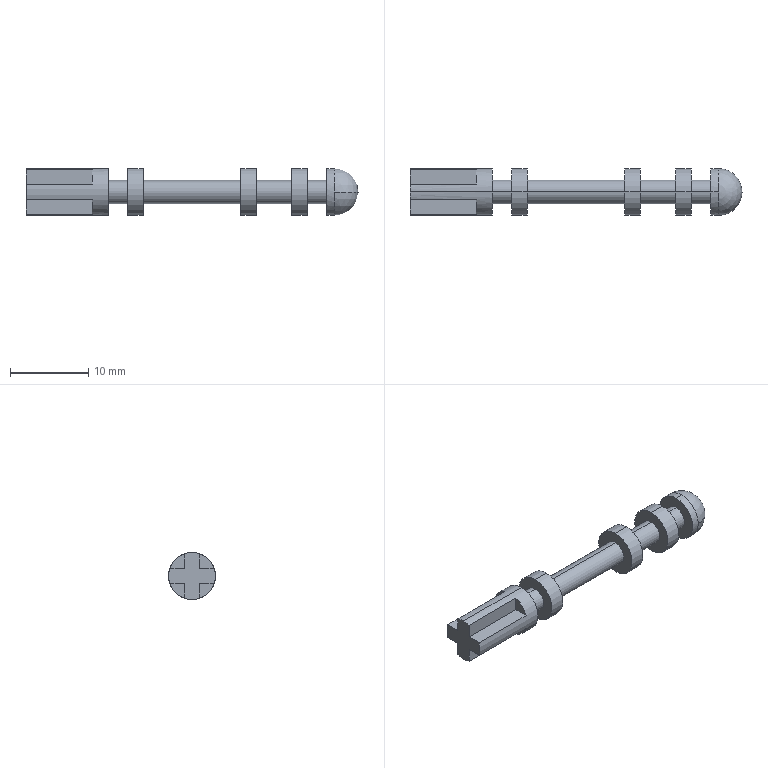Part | SolidWorks | features ICE 1, Revolution 1 | 1 solid | 41 faces | box 42.5 x 6 x 6 mm | volume 632.683 mm3 | plane 21 | cylinder 18 | sphere 2 | commonest cylinder face diameters 6 x10 3 x8
STEP:
#1=CARTESIAN_POINT('',(42.5,0.,0.));
#2=VERTEX_POINT('',#1);
#3=CARTESIAN_POINT('',(39.5,3.,0.));
#4=VERTEX_POINT('',#3);
#5=CARTESIAN_POINT('',(39.5,0.,0.));
#6=DIRECTION('',(0.,0.,1.));
#7=DIRECTION('',(1.,0.,0.));
#8=AXIS2_PLACEMENT_3D('',#5,#6,#7);
#9=CIRCLE('',#8,3.);
#10=EDGE_CURVE('',#2,#4,#9,.T.);
#11=ORIENTED_EDGE('',*,*,#10,.F.);
#12=CARTESIAN_POINT('',(39.5,-3.,0.));
#13=VERTEX_POINT('',#12);
#14=CARTESIAN_POINT('',(39.5,0.,0.));
#15=DIRECTION('',(0.,0.,-1.));
#16=DIRECTION('',(0.,1.,0.));
#17=AXIS2_PLACEMENT_3D('',#14,#15,#16);
#18=CIRCLE('',#17,3.);
#19=EDGE_CURVE('',#2,#13,#18,.T.);
#20=ORIENTED_EDGE('',*,*,#19,.T.);
#21=CARTESIAN_POINT('',(39.5,0.,-3.));
#22=VERTEX_POINT('',#21);
#23=CARTESIAN_POINT('',(39.5,0.,0.));
#24=DIRECTION('',(-1.,0.,0.));
#25=DIRECTION('',(0.,0.,1.));
#26=AXIS2_PLACEMENT_3D('',#23,#24,#25);
#27=CIRCLE('',#26,3.);
#28=EDGE_CURVE('',#22,#13,#27,.T.);
#29=ORIENTED_EDGE('',*,*,#28,.F.);
#30=CARTESIAN_POINT('',(39.5,0.,0.));
#31=DIRECTION('',(-1.,0.,0.));
#32=DIRECTION('',(0.,0.,1.));
#33=AXIS2_PLACEMENT_3D('',#30,#31,#32);
#34=CIRCLE('',#33,3.);
#35=EDGE_CURVE('',#4,#22,#34,.T.);
#36=ORIENTED_EDGE('',*,*,#35,.F.);
#37=EDGE_LOOP('',(#11,#20,#29,#36));
#38=FACE_OUTER_BOUND('',#37,.T.);
#39=CARTESIAN_POINT('',(39.5,0.,0.));
#40=DIRECTION('',(0.,0.,-1.));
#41=DIRECTION('',(0.,1.,0.));
#42=AXIS2_PLACEMENT_3D('',#39,#40,#41);
#43=SPHERICAL_SURFACE('',#42,3.);
#44=ADVANCED_FACE('',(#38),#43,.T.);
#45=CARTESIAN_POINT('',(39.5,0.,3.));
#46=VERTEX_POINT('',#45);
#47=CARTESIAN_POINT('',(39.5,0.,0.));
#48=DIRECTION('',(-1.,0.,0.));
#49=DIRECTION('',(0.,0.,1.));
#50=AXIS2_PLACEMENT_3D('',#47,#48,#49);
#51=CIRCLE('',#50,3.);
#52=EDGE_CURVE('',#46,#4,#51,.T.);
#53=ORIENTED_EDGE('',*,*,#52,.T.);
#54=ORIENTED_EDGE('',*,*,#35,.T.);
#55=CARTESIAN_POINT('',(38.5,0.,-3.));
#56=VERTEX_POINT('',#55);
#57=CARTESIAN_POINT('',(0.,0.,-3.));
#58=DIRECTION('',(-1.,0.,0.));
#59=VECTOR('',#58,1000.);
#60=LINE('',#57,#59);
#61=EDGE_CURVE('',#22,#56,#60,.T.);
#62=ORIENTED_EDGE('',*,*,#61,.T.);
#63=CARTESIAN_POINT('',(38.5,0.,3.));
#64=VERTEX_POINT('',#63);
#65=CARTESIAN_POINT('',(38.5,0.,0.));
#66=DIRECTION('',(-1.,0.,0.));
#67=DIRECTION('',(0.,0.,1.));
#68=AXIS2_PLACEMENT_3D('',#65,#66,#67);
#69=CIRCLE('',#68,3.);
#70=EDGE_CURVE('',#64,#56,#69,.T.);
#71=ORIENTED_EDGE('',*,*,#70,.F.);
#72=CARTESIAN_POINT('',(0.,0.,3.));
#73=DIRECTION('',(-1.,0.,0.));
#74=VECTOR('',#73,1000.);
#75=LINE('',#72,#74);
#76=EDGE_CURVE('',#46,#64,#75,.T.);
#77=ORIENTED_EDGE('',*,*,#76,.F.);
#78=EDGE_LOOP('',(#53,#54,#62,#71,#77));
#79=FACE_OUTER_BOUND('',#78,.T.);
#80=CARTESIAN_POINT('',(0.,0.,0.));
#81=DIRECTION('',(-1.,0.,0.));
#82=DIRECTION('',(0.,0.,1.));
#83=AXIS2_PLACEMENT_3D('',#80,#81,#82);
#84=CYLINDRICAL_SURFACE('',#83,3.);
#85=ADVANCED_FACE('',(#79),#84,.T.);
#86=CARTESIAN_POINT('',(38.5,0.,1.5));
#87=VERTEX_POINT('',#86);
#88=CARTESIAN_POINT('',(38.5,0.,-1.5));
#89=VERTEX_POINT('',#88);
#90=CARTESIAN_POINT('',(38.5,0.,0.));
#91=DIRECTION('',(-1.,0.,0.));
#92=DIRECTION('',(0.,0.,1.));
#93=AXIS2_PLACEMENT_3D('',#90,#91,#92);
#94=CIRCLE('',#93,1.5);
#95=EDGE_CURVE('',#87,#89,#94,.T.);
#96=ORIENTED_EDGE('',*,*,#95,.T.);
#97=CARTESIAN_POINT('',(36.,0.,-1.5));
#98=VERTEX_POINT('',#97);
#99=CARTESIAN_POINT('',(0.,0.,-1.5));
#100=DIRECTION('',(-1.,0.,0.));
#101=VECTOR('',#100,1000.);
#102=LINE('',#99,#101);
#103=EDGE_CURVE('',#89,#98,#102,.T.);
#104=ORIENTED_EDGE('',*,*,#103,.T.);
#105=CARTESIAN_POINT('',(36.,0.,1.5));
#106=VERTEX_POINT('',#105);
#107=CARTESIAN_POINT('',(36.,0.,0.));
#108=DIRECTION('',(-1.,0.,0.));
#109=DIRECTION('',(0.,0.,1.));
#110=AXIS2_PLACEMENT_3D('',#107,#108,#109);
#111=CIRCLE('',#110,1.5);
#112=EDGE_CURVE('',#106,#98,#111,.T.);
#113=ORIENTED_EDGE('',*,*,#112,.F.);
#114=CARTESIAN_POINT('',(0.,0.,1.5));
#115=DIRECTION('',(-1.,0.,0.));
#116=VECTOR('',#115,1000.);
#117=LINE('',#114,#116);
#118=EDGE_CURVE('',#87,#106,#117,.T.);
#119=ORIENTED_EDGE('',*,*,#118,.F.);
#120=EDGE_LOOP('',(#96,#104,#113,#119));
#121=FACE_OUTER_BOUND('',#120,.T.);
#122=CARTESIAN_POINT('',(0.,0.,0.));
#123=DIRECTION('',(-1.,0.,0.));
#124=DIRECTION('',(0.,0.,1.));
#125=AXIS2_PLACEMENT_3D('',#122,#123,#124);
#126=CYLINDRICAL_SURFACE('',#125,1.5);
#127=ADVANCED_FACE('',(#121),#126,.T.);
#128=CARTESIAN_POINT('',(36.,0.,3.));
#129=VERTEX_POINT('',#128);
#130=CARTESIAN_POINT('',(36.,0.,-3.));
#131=VERTEX_POINT('',#130);
#132=CARTESIAN_POINT('',(36.,0.,0.));
#133=DIRECTION('',(-1.,0.,0.));
#134=DIRECTION('',(0.,0.,1.));
#135=AXIS2_PLACEMENT_3D('',#132,#133,#134);
#136=CIRCLE('',#135,3.);
#137=EDGE_CURVE('',#129,#131,#136,.T.);
#138=ORIENTED_EDGE('',*,*,#137,.T.);
#139=CARTESIAN_POINT('',(34.,0.,-3.));
#140=VERTEX_POINT('',#139);
#141=CARTESIAN_POINT('',(0.,0.,-3.));
#142=DIRECTION('',(-1.,0.,0.));
#143=VECTOR('',#142,1000.);
#144=LINE('',#141,#143);
#145=EDGE_CURVE('',#131,#140,#144,.T.);
#146=ORIENTED_EDGE('',*,*,#145,.T.);
#147=CARTESIAN_POINT('',(34.,0.,3.));
#148=VERTEX_POINT('',#147);
#149=CARTESIAN_POINT('',(34.,0.,0.));
#150=DIRECTION('',(-1.,0.,0.));
#151=DIRECTION('',(0.,0.,1.));
#152=AXIS2_PLACEMENT_3D('',#149,#150,#151);
#153=CIRCLE('',#152,3.);
#154=EDGE_CURVE('',#148,#140,#153,.T.);
#155=ORIENTED_EDGE('',*,*,#154,.F.);
#156=CARTESIAN_POINT('',(0.,0.,3.));
#157=DIRECTION('',(-1.,0.,0.));
#158=VECTOR('',#157,1000.);
#159=LINE('',#156,#158);
#160=EDGE_CURVE('',#129,#148,#159,.T.);
#161=ORIENTED_EDGE('',*,*,#160,.F.);
#162=EDGE_LOOP('',(#138,#146,#155,#161));
#163=FACE_OUTER_BOUND('',#162,.T.);
#164=CARTESIAN_POINT('',(0.,0.,0.));
#165=DIRECTION('',(-1.,0.,0.));
#166=DIRECTION('',(0.,0.,1.));
#167=AXIS2_PLACEMENT_3D('',#164,#165,#166);
#168=CYLINDRICAL_SURFACE('',#167,3.);
#169=ADVANCED_FACE('',(#163),#168,.T.);
#170=CARTESIAN_POINT('',(34.,0.,1.5));
#171=VERTEX_POINT('',#170);
#172=CARTESIAN_POINT('',(34.,0.,-1.5));
#173=VERTEX_POINT('',#172);
#174=CARTESIAN_POINT('',(34.,0.,0.));
#175=DIRECTION('',(-1.,0.,0.));
#176=DIRECTION('',(0.,0.,1.));
#177=AXIS2_PLACEMENT_3D('',#174,#175,#176);
#178=CIRCLE('',#177,1.5);
#179=EDGE_CURVE('',#171,#173,#178,.T.);
#180=ORIENTED_EDGE('',*,*,#179,.T.);
#181=CARTESIAN_POINT('',(29.5,0.,-1.5));
#182=VERTEX_POINT('',#181);
#183=CARTESIAN_POINT('',(0.,0.,-1.5));
#184=DIRECTION('',(-1.,0.,0.));
#185=VECTOR('',#184,1000.);
#186=LINE('',#183,#185);
#187=EDGE_CURVE('',#173,#182,#186,.T.);
#188=ORIENTED_EDGE('',*,*,#187,.T.);
#189=CARTESIAN_POINT('',(29.5,0.,1.5));
#190=VERTEX_POINT('',#189);
#191=CARTESIAN_POINT('',(29.5,0.,0.));
#192=DIRECTION('',(-1.,0.,0.));
#193=DIRECTION('',(0.,0.,1.));
#194=AXIS2_PLACEMENT_3D('',#191,#192,#193);
#195=CIRCLE('',#194,1.5);
#196=EDGE_CURVE('',#190,#182,#195,.T.);
#197=ORIENTED_EDGE('',*,*,#196,.F.);
#198=CARTESIAN_POINT('',(0.,0.,1.5));
#199=DIRECTION('',(-1.,0.,0.));
#200=VECTOR('',#199,1000.);
#201=LINE('',#198,#200);
#202=EDGE_CURVE('',#171,#190,#201,.T.);
#203=ORIENTED_EDGE('',*,*,#202,.F.);
#204=EDGE_LOOP('',(#180,#188,#197,#203));
#205=FACE_OUTER_BOUND('',#204,.T.);
#206=CARTESIAN_POINT('',(0.,0.,0.));
#207=DIRECTION('',(-1.,0.,0.));
#208=DIRECTION('',(0.,0.,1.));
#209=AXIS2_PLACEMENT_3D('',#206,#207,#208);
#210=CYLINDRICAL_SURFACE('',#209,1.5);
#211=ADVANCED_FACE('',(#205),#210,.T.);
#212=CARTESIAN_POINT('',(29.5,0.,3.));
#213=VERTEX_POINT('',#212);
#214=CARTESIAN_POINT('',(29.5,0.,-3.));
#215=VERTEX_POINT('',#214);
#216=CARTESIAN_POINT('',(29.5,0.,0.));
#217=DIRECTION('',(-1.,0.,0.));
#218=DIRECTION('',(0.,0.,1.));
#219=AXIS2_PLACEMENT_3D('',#216,#217,#218);
#220=CIRCLE('',#219,3.);
#221=EDGE_CURVE('',#213,#215,#220,.T.);
#222=ORIENTED_EDGE('',*,*,#221,.T.);
#223=CARTESIAN_POINT('',(27.5,0.,-3.));
#224=VERTEX_POINT('',#223);
#225=CARTESIAN_POINT('',(0.,0.,-3.));
#226=DIRECTION('',(-1.,0.,0.));
#227=VECTOR('',#226,1000.);
#228=LINE('',#225,#227);
#229=EDGE_CURVE('',#215,#224,#228,.T.);
#230=ORIENTED_EDGE('',*,*,#229,.T.);
#231=CARTESIAN_POINT('',(27.5,0.,3.));
#232=VERTEX_POINT('',#231);
#233=CARTESIAN_POINT('',(27.5,0.,0.));
#234=DIRECTION('',(-1.,0.,0.));
#235=DIRECTION('',(0.,0.,1.));
#236=AXIS2_PLACEMENT_3D('',#233,#234,#235);
#237=CIRCLE('',#236,3.);
#238=EDGE_CURVE('',#232,#224,#237,.T.);
#239=ORIENTED_EDGE('',*,*,#238,.F.);
#240=CARTESIAN_POINT('',(0.,0.,3.));
#241=DIRECTION('',(-1.,0.,0.));
#242=VECTOR('',#241,1000.);
#243=LINE('',#240,#242);
#244=EDGE_CURVE('',#213,#232,#243,.T.);
#245=ORIENTED_EDGE('',*,*,#244,.F.);
#246=EDGE_LOOP('',(#222,#230,#239,#245));
#247=FACE_OUTER_BOUND('',#246,.T.);
#248=CARTESIAN_POINT('',(0.,0.,0.));
#249=DIRECTION('',(-1.,0.,0.));
#250=DIRECTION('',(0.,0.,1.));
#251=AXIS2_PLACEMENT_3D('',#248,#249,#250);
#252=CYLINDRICAL_SURFACE('',#251,3.);
#253=ADVANCED_FACE('',(#247),#252,.T.);
#254=CARTESIAN_POINT('',(27.5,0.,1.5));
#255=VERTEX_POINT('',#254);
#256=CARTESIAN_POINT('',(27.5,0.,-1.5));
#257=VERTEX_POINT('',#256);
#258=CARTESIAN_POINT('',(27.5,0.,0.));
#259=DIRECTION('',(-1.,0.,0.));
#260=DIRECTION('',(0.,0.,1.));
#261=AXIS2_PLACEMENT_3D('',#258,#259,#260);
#262=CIRCLE('',#261,1.5);
#263=EDGE_CURVE('',#255,#257,#262,.T.);
#264=ORIENTED_EDGE('',*,*,#263,.T.);
#265=CARTESIAN_POINT('',(15.,0.,-1.5));
#266=VERTEX_POINT('',#265);
#267=CARTESIAN_POINT('',(0.,0.,-1.5));
#268=DIRECTION('',(-1.,0.,0.));
#269=VECTOR('',#268,1000.);
#270=LINE('',#267,#269);
#271=EDGE_CURVE('',#257,#266,#270,.T.);
#272=ORIENTED_EDGE('',*,*,#271,.T.);
#273=CARTESIAN_POINT('',(15.,0.,1.5));
#274=VERTEX_POINT('',#273);
#275=CARTESIAN_POINT('',(15.,0.,0.));
#276=DIRECTION('',(-1.,0.,0.));
#277=DIRECTION('',(0.,0.,1.));
#278=AXIS2_PLACEMENT_3D('',#275,#276,#277);
#279=CIRCLE('',#278,1.5);
#280=EDGE_CURVE('',#274,#266,#279,.T.);
#281=ORIENTED_EDGE('',*,*,#280,.F.);
#282=CARTESIAN_POINT('',(0.,0.,1.5));
#283=DIRECTION('',(-1.,0.,0.));
#284=VECTOR('',#283,1000.);
#285=LINE('',#282,#284);
#286=EDGE_CURVE('',#255,#274,#285,.T.);
#287=ORIENTED_EDGE('',*,*,#286,.F.);
#288=EDGE_LOOP('',(#264,#272,#281,#287));
#289=FACE_OUTER_BOUND('',#288,.T.);
#290=CARTESIAN_POINT('',(0.,0.,0.));
#291=DIRECTION('',(-1.,0.,0.));
#292=DIRECTION('',(0.,0.,1.));
#293=AXIS2_PLACEMENT_3D('',#290,#291,#292);
#294=CYLINDRICAL_SURFACE('',#293,1.5);
#295=ADVANCED_FACE('',(#289),#294,.T.);
#296=CARTESIAN_POINT('',(15.,0.,3.));
#297=VERTEX_POINT('',#296);
#298=CARTESIAN_POINT('',(15.,0.,-3.));
#299=VERTEX_POINT('',#298);
#300=CARTESIAN_POINT('',(15.,0.,0.));
#301=DIRECTION('',(-1.,0.,0.));
#302=DIRECTION('',(0.,0.,1.));
#303=AXIS2_PLACEMENT_3D('',#300,#301,#302);
#304=CIRCLE('',#303,3.);
#305=EDGE_CURVE('',#297,#299,#304,.T.);
#306=ORIENTED_EDGE('',*,*,#305,.T.);
#307=CARTESIAN_POINT('',(13.,0.,-3.));
#308=VERTEX_POINT('',#307);
#309=CARTESIAN_POINT('',(0.,0.,-3.));
#310=DIRECTION('',(-1.,0.,0.));
#311=VECTOR('',#310,1000.);
#312=LINE('',#309,#311);
#313=EDGE_CURVE('',#299,#308,#312,.T.);
#314=ORIENTED_EDGE('',*,*,#313,.T.);
#315=CARTESIAN_POINT('',(13.,0.,3.));
#316=VERTEX_POINT('',#315);
#317=CARTESIAN_POINT('',(13.,0.,0.));
#318=DIRECTION('',(-1.,0.,0.));
#319=DIRECTION('',(0.,0.,1.));
#320=AXIS2_PLACEMENT_3D('',#317,#318,#319);
#321=CIRCLE('',#320,3.);
#322=EDGE_CURVE('',#316,#308,#321,.T.);
#323=ORIENTED_EDGE('',*,*,#322,.F.);
#324=CARTESIAN_POINT('',(0.,0.,3.));
#325=DIRECTION('',(-1.,0.,0.));
#326=VECTOR('',#325,1000.);
#327=LINE('',#324,#326);
#328=EDGE_CURVE('',#297,#316,#327,.T.);
#329=ORIENTED_EDGE('',*,*,#328,.F.);
#330=EDGE_LOOP('',(#306,#314,#323,#329));
#331=FACE_OUTER_BOUND('',#330,.T.);
#332=CARTESIAN_POINT('',(0.,0.,0.));
#333=DIRECTION('',(-1.,0.,0.));
#334=DIRECTION('',(0.,0.,1.));
#335=AXIS2_PLACEMENT_3D('',#332,#333,#334);
#336=CYLINDRICAL_SURFACE('',#335,3.);
#337=ADVANCED_FACE('',(#331),#336,.T.);
#338=CARTESIAN_POINT('',(13.,0.,1.5));
#339=VERTEX_POINT('',#338);
#340=CARTESIAN_POINT('',(13.,0.,-1.5));
#341=VERTEX_POINT('',#340);
#342=CARTESIAN_POINT('',(13.,0.,0.));
#343=DIRECTION('',(-1.,0.,0.));
#344=DIRECTION('',(0.,0.,1.));
#345=AXIS2_PLACEMENT_3D('',#342,#343,#344);
#346=CIRCLE('',#345,1.5);
#347=EDGE_CURVE('',#339,#341,#346,.T.);
#348=ORIENTED_EDGE('',*,*,#347,.T.);
#349=CARTESIAN_POINT('',(10.5,0.,-1.5));
#350=VERTEX_POINT('',#349);
#351=CARTESIAN_POINT('',(0.,0.,-1.5));
#352=DIRECTION('',(-1.,0.,0.));
#353=VECTOR('',#352,1000.);
#354=LINE('',#351,#353);
#355=EDGE_CURVE('',#341,#350,#354,.T.);
#356=ORIENTED_EDGE('',*,*,#355,.T.);
#357=CARTESIAN_POINT('',(10.5,0.,1.5));
#358=VERTEX_POINT('',#357);
#359=CARTESIAN_POINT('',(10.5,0.,0.));
#360=DIRECTION('',(-1.,0.,0.));
#361=DIRECTION('',(0.,0.,1.));
#362=AXIS2_PLACEMENT_3D('',#359,#360,#361);
#363=CIRCLE('',#362,1.5);
#364=EDGE_CURVE('',#358,#350,#363,.T.);
#365=ORIENTED_EDGE('',*,*,#364,.F.);
#366=CARTESIAN_POINT('',(0.,0.,1.5));
#367=DIRECTION('',(-1.,0.,0.));
#368=VECTOR('',#367,1000.);
#369=LINE('',#366,#368);
#370=EDGE_CURVE('',#339,#358,#369,.T.);
#371=ORIENTED_EDGE('',*,*,#370,.F.);
#372=EDGE_LOOP('',(#348,#356,#365,#371));
#373=FACE_OUTER_BOUND('',#372,.T.);
#374=CARTESIAN_POINT('',(0.,0.,0.));
#375=DIRECTION('',(-1.,0.,0.));
#376=DIRECTION('',(0.,0.,1.));
#377=AXIS2_PLACEMENT_3D('',#374,#375,#376);
#378=CYLINDRICAL_SURFACE('',#377,1.5);
#379=ADVANCED_FACE('',(#373),#378,.T.);
#380=CARTESIAN_POINT('',(10.5,0.,3.));
#381=VERTEX_POINT('',#380);
#382=CARTESIAN_POINT('',(10.5,0.,-3.));
#383=VERTEX_POINT('',#382);
#384=CARTESIAN_POINT('',(10.5,0.,0.));
#385=DIRECTION('',(-1.,0.,0.));
#386=DIRECTION('',(0.,0.,1.));
#387=AXIS2_PLACEMENT_3D('',#384,#385,#386);
#388=CIRCLE('',#387,3.);
#389=EDGE_CURVE('',#381,#383,#388,.T.);
#390=ORIENTED_EDGE('',*,*,#389,.T.);
#391=CARTESIAN_POINT('',(0.,0.,-3.));
#392=VERTEX_POINT('',#391);
#393=CARTESIAN_POINT('',(0.,0.,-3.));
#394=DIRECTION('',(-1.,0.,0.));
#395=VECTOR('',#394,1000.);
#396=LINE('',#393,#395);
#397=EDGE_CURVE('',#383,#392,#396,.T.);
#398=ORIENTED_EDGE('',*,*,#397,.T.);
#399=CARTESIAN_POINT('',(0.,1.,-2.828));
#400=VERTEX_POINT('',#399);
#401=CARTESIAN_POINT('',(0.,0.,0.));
#402=DIRECTION('',(-1.,0.,0.));
#403=DIRECTION('',(0.,0.,1.));
#404=AXIS2_PLACEMENT_3D('',#401,#402,#403);
#405=CIRCLE('',#404,3.);
#406=EDGE_CURVE('',#400,#392,#405,.T.);
#407=ORIENTED_EDGE('',*,*,#406,.F.);
#408=CARTESIAN_POINT('',(8.5,1.,-2.828));
#409=VERTEX_POINT('',#408);
#410=CARTESIAN_POINT('',(8.5,1.,-2.828));
#411=DIRECTION('',(-1.,0.,0.));
#412=VECTOR('',#411,1000.);
#413=LINE('',#410,#412);
#414=EDGE_CURVE('',#409,#400,#413,.T.);
#415=ORIENTED_EDGE('',*,*,#414,.F.);
#416=CARTESIAN_POINT('',(8.5,2.828,-1.));
#417=VERTEX_POINT('',#416);
#418=CARTESIAN_POINT('',(8.5,0.,0.));
#419=DIRECTION('',(-1.,0.,0.));
#420=DIRECTION('',(0.,0.,1.));
#421=AXIS2_PLACEMENT_3D('',#418,#419,#420);
#422=CIRCLE('',#421,3.);
#423=EDGE_CURVE('',#417,#409,#422,.T.);
#424=ORIENTED_EDGE('',*,*,#423,.F.);
#425=CARTESIAN_POINT('',(0.,2.828,-1.));
#426=VERTEX_POINT('',#425);
#427=CARTESIAN_POINT('',(8.5,2.828,-1.));
#428=DIRECTION('',(-1.,0.,0.));
#429=VECTOR('',#428,1000.);
#430=LINE('',#427,#429);
#431=EDGE_CURVE('',#417,#426,#430,.T.);
#432=ORIENTED_EDGE('',*,*,#431,.T.);
#433=CARTESIAN_POINT('',(0.,2.828,1.));
#434=VERTEX_POINT('',#433);
#435=CARTESIAN_POINT('',(0.,0.,0.));
#436=DIRECTION('',(-1.,0.,0.));
#437=DIRECTION('',(0.,0.,1.));
#438=AXIS2_PLACEMENT_3D('',#435,#436,#437);
#439=CIRCLE('',#438,3.);
#440=EDGE_CURVE('',#434,#426,#439,.T.);
#441=ORIENTED_EDGE('',*,*,#440,.F.);
#442=CARTESIAN_POINT('',(8.5,2.828,1.));
#443=VERTEX_POINT('',#442);
#444=CARTESIAN_POINT('',(8.5,2.828,1.));
#445=DIRECTION('',(-1.,0.,0.));
#446=VECTOR('',#445,1000.);
#447=LINE('',#444,#446);
#448=EDGE_CURVE('',#443,#434,#447,.T.);
#449=ORIENTED_EDGE('',*,*,#448,.F.);
#450=CARTESIAN_POINT('',(8.5,1.,2.828));
#451=VERTEX_POINT('',#450);
#452=CARTESIAN_POINT('',(8.5,0.,0.));
#453=DIRECTION('',(-1.,0.,0.));
#454=DIRECTION('',(0.,0.,1.));
#455=AXIS2_PLACEMENT_3D('',#452,#453,#454);
#456=CIRCLE('',#455,3.);
#457=EDGE_CURVE('',#451,#443,#456,.T.);
#458=ORIENTED_EDGE('',*,*,#457,.F.);
#459=CARTESIAN_POINT('',(0.,1.,2.828));
#460=VERTEX_POINT('',#459);
#461=CARTESIAN_POINT('',(8.5,1.,2.828));
#462=DIRECTION('',(-1.,0.,0.));
#463=VECTOR('',#462,1000.);
#464=LINE('',#461,#463);
#465=EDGE_CURVE('',#451,#460,#464,.T.);
#466=ORIENTED_EDGE('',*,*,#465,.T.);
#467=CARTESIAN_POINT('',(0.,0.,3.));
#468=VERTEX_POINT('',#467);
#469=CARTESIAN_POINT('',(0.,0.,0.));
#470=DIRECTION('',(-1.,0.,0.));
#471=DIRECTION('',(0.,0.,1.));
#472=AXIS2_PLACEMENT_3D('',#469,#470,#471);
#473=CIRCLE('',#472,3.);
#474=EDGE_CURVE('',#468,#460,#473,.T.);
#475=ORIENTED_EDGE('',*,*,#474,.F.);
#476=CARTESIAN_POINT('',(0.,0.,3.));
#477=DIRECTION('',(-1.,0.,0.));
#478=VECTOR('',#477,1000.);
#479=LINE('',#476,#478);
#480=EDGE_CURVE('',#381,#468,#479,.T.);
#481=ORIENTED_EDGE('',*,*,#480,.F.);
#482=EDGE_LOOP('',(#390,#398,#407,#415,#424,#432,#441,#449,#458,#466,#475,#481));
#483=FACE_OUTER_BOUND('',#482,.T.);
#484=CARTESIAN_POINT('',(0.,0.,0.));
#485=DIRECTION('',(-1.,0.,0.));
#486=DIRECTION('',(0.,0.,1.));
#487=AXIS2_PLACEMENT_3D('',#484,#485,#486);
#488=CYLINDRICAL_SURFACE('',#487,3.);
#489=ADVANCED_FACE('',(#483),#488,.T.);
#490=CARTESIAN_POINT('',(0.,-1.,1.));
#491=VERTEX_POINT('',#490);
#492=CARTESIAN_POINT('',(0.,-1.,2.828));
#493=VERTEX_POINT('',#492);
#494=CARTESIAN_POINT('',(0.,-1.,0.));
#495=DIRECTION('',(0.,0.,1.));
#496=VECTOR('',#495,1000.);
#497=LINE('',#494,#496);
#498=EDGE_CURVE('',#491,#493,#497,.T.);
#499=ORIENTED_EDGE('',*,*,#498,.T.);
#500=CARTESIAN_POINT('',(0.,0.,0.));
#501=DIRECTION('',(-1.,0.,0.));
#502=DIRECTION('',(0.,0.,1.));
#503=AXIS2_PLACEMENT_3D('',#500,#501,#502);
#504=CIRCLE('',#503,3.);
#505=EDGE_CURVE('',#493,#468,#504,.T.);
#506=ORIENTED_EDGE('',*,*,#505,.T.);
#507=ORIENTED_EDGE('',*,*,#474,.T.);
#508=CARTESIAN_POINT('',(0.,1.,1.));
#509=VERTEX_POINT('',#508);
#510=CARTESIAN_POINT('',(0.,1.,0.));
#511=DIRECTION('',(0.,0.,1.));
#512=VECTOR('',#511,1000.);
#513=LINE('',#510,#512);
#514=EDGE_CURVE('',#509,#460,#513,.T.);
#515=ORIENTED_EDGE('',*,*,#514,.F.);
#516=CARTESIAN_POINT('',(0.,0.,1.));
#517=DIRECTION('',(0.,1.,0.));
#518=VECTOR('',#517,1000.);
#519=LINE('',#516,#518);
#520=EDGE_CURVE('',#509,#434,#519,.T.);
#521=ORIENTED_EDGE('',*,*,#520,.T.);
#522=ORIENTED_EDGE('',*,*,#440,.T.);
#523=CARTESIAN_POINT('',(0.,1.,-1.));
#524=VERTEX_POINT('',#523);
#525=CARTESIAN_POINT('',(0.,0.,-1.));
#526=DIRECTION('',(0.,1.,0.));
#527=VECTOR('',#526,1000.);
#528=LINE('',#525,#527);
#529=EDGE_CURVE('',#524,#426,#528,.T.);
#530=ORIENTED_EDGE('',*,*,#529,.F.);
#531=CARTESIAN_POINT('',(0.,1.,0.));
#532=DIRECTION('',(0.,0.,1.));
#533=VECTOR('',#532,1000.);
#534=LINE('',#531,#533);
#535=EDGE_CURVE('',#400,#524,#534,.T.);
#536=ORIENTED_EDGE('',*,*,#535,.F.);
#537=ORIENTED_EDGE('',*,*,#406,.T.);
#538=CARTESIAN_POINT('',(0.,-1.,-2.828));
#539=VERTEX_POINT('',#538);
#540=CARTESIAN_POINT('',(0.,0.,0.));
#541=DIRECTION('',(-1.,0.,0.));
#542=DIRECTION('',(0.,0.,1.));
#543=AXIS2_PLACEMENT_3D('',#540,#541,#542);
#544=CIRCLE('',#543,3.);
#545=EDGE_CURVE('',#392,#539,#544,.T.);
#546=ORIENTED_EDGE('',*,*,#545,.T.);
#547=CARTESIAN_POINT('',(0.,-1.,-1.));
#548=VERTEX_POINT('',#547);
#549=CARTESIAN_POINT('',(0.,-1.,0.));
#550=DIRECTION('',(0.,0.,1.));
#551=VECTOR('',#550,1000.);
#552=LINE('',#549,#551);
#553=EDGE_CURVE('',#539,#548,#552,.T.);
#554=ORIENTED_EDGE('',*,*,#553,.T.);
#555=CARTESIAN_POINT('',(0.,-2.828,-1.));
#556=VERTEX_POINT('',#555);
#557=CARTESIAN_POINT('',(0.,0.,-1.));
#558=DIRECTION('',(0.,1.,0.));
#559=VECTOR('',#558,1000.);
#560=LINE('',#557,#559);
#561=EDGE_CURVE('',#556,#548,#560,.T.);
#562=ORIENTED_EDGE('',*,*,#561,.F.);
#563=CARTESIAN_POINT('',(0.,-2.828,1.));
#564=VERTEX_POINT('',#563);
#565=CARTESIAN_POINT('',(0.,0.,0.));
#566=DIRECTION('',(-1.,0.,0.));
#567=DIRECTION('',(0.,0.,1.));
#568=AXIS2_PLACEMENT_3D('',#565,#566,#567);
#569=CIRCLE('',#568,3.);
#570=EDGE_CURVE('',#556,#564,#569,.T.);
#571=ORIENTED_EDGE('',*,*,#570,.T.);
#572=CARTESIAN_POINT('',(0.,0.,1.));
#573=DIRECTION('',(0.,1.,0.));
#574=VECTOR('',#573,1000.);
#575=LINE('',#572,#574);
#576=EDGE_CURVE('',#564,#491,#575,.T.);
#577=ORIENTED_EDGE('',*,*,#576,.T.);
#578=EDGE_LOOP('',(#499,#506,#507,#515,#521,#522,#530,#536,#537,#546,#554,#562,#571,#577));
#579=FACE_OUTER_BOUND('',#578,.T.);
#580=CARTESIAN_POINT('',(0.,0.,0.));
#581=DIRECTION('',(1.,0.,0.));
#582=DIRECTION('',(0.,0.,-1.));
#583=AXIS2_PLACEMENT_3D('',#580,#581,#582);
#584=PLANE('',#583);
#585=ADVANCED_FACE('',(#579),#584,.F.);
#586=ORIENTED_EDGE('',*,*,#397,.F.);
#587=CARTESIAN_POINT('',(10.5,0.,0.));
#588=DIRECTION('',(-1.,0.,0.));
#589=DIRECTION('',(0.,0.,1.));
#590=AXIS2_PLACEMENT_3D('',#587,#588,#589);
#591=CIRCLE('',#590,3.);
#592=EDGE_CURVE('',#383,#381,#591,.T.);
#593=ORIENTED_EDGE('',*,*,#592,.T.);
#594=ORIENTED_EDGE('',*,*,#480,.T.);
#595=ORIENTED_EDGE('',*,*,#505,.F.);
#596=CARTESIAN_POINT('',(8.5,-1.,2.828));
#597=VERTEX_POINT('',#596);
#598=CARTESIAN_POINT('',(8.5,-1.,2.828));
#599=DIRECTION('',(-1.,0.,0.));
#600=VECTOR('',#599,1000.);
#601=LINE('',#598,#600);
#602=EDGE_CURVE('',#597,#493,#601,.T.);
#603=ORIENTED_EDGE('',*,*,#602,.F.);
#604=CARTESIAN_POINT('',(8.5,-2.828,1.));
#605=VERTEX_POINT('',#604);
#606=CARTESIAN_POINT('',(8.5,0.,0.));
#607=DIRECTION('',(-1.,0.,0.));
#608=DIRECTION('',(0.,0.,1.));
#609=AXIS2_PLACEMENT_3D('',#606,#607,#608);
#610=CIRCLE('',#609,3.);
#611=EDGE_CURVE('',#605,#597,#610,.T.);
#612=ORIENTED_EDGE('',*,*,#611,.F.);
#613=CARTESIAN_POINT('',(8.5,-2.828,1.));
#614=DIRECTION('',(-1.,0.,0.));
#615=VECTOR('',#614,1000.);
#616=LINE('',#613,#615);
#617=EDGE_CURVE('',#605,#564,#616,.T.);
#618=ORIENTED_EDGE('',*,*,#617,.T.);
#619=ORIENTED_EDGE('',*,*,#570,.F.);
#620=CARTESIAN_POINT('',(8.5,-2.828,-1.));
#621=VERTEX_POINT('',#620);
#622=CARTESIAN_POINT('',(8.5,-2.828,-1.));
#623=DIRECTION('',(-1.,0.,0.));
#624=VECTOR('',#623,1000.);
#625=LINE('',#622,#624);
#626=EDGE_CURVE('',#621,#556,#625,.T.);
#627=ORIENTED_EDGE('',*,*,#626,.F.);
#628=CARTESIAN_POINT('',(8.5,-1.,-2.828));
#629=VERTEX_POINT('',#628);
#630=CARTESIAN_POINT('',(8.5,0.,0.));
#631=DIRECTION('',(-1.,0.,0.));
#632=DIRECTION('',(0.,0.,1.));
#633=AXIS2_PLACEMENT_3D('',#630,#631,#632);
#634=CIRCLE('',#633,3.);
#635=EDGE_CURVE('',#629,#621,#634,.T.);
#636=ORIENTED_EDGE('',*,*,#635,.F.);
#637=CARTESIAN_POINT('',(8.5,-1.,-2.828));
#638=DIRECTION('',(-1.,0.,0.));
#639=VECTOR('',#638,1000.);
#640=LINE('',#637,#639);
#641=EDGE_CURVE('',#629,#539,#640,.T.);
#642=ORIENTED_EDGE('',*,*,#641,.T.);
#643=ORIENTED_EDGE('',*,*,#545,.F.);
#644=EDGE_LOOP('',(#586,#593,#594,#595,#603,#612,#618,#619,#627,#636,#642,#643));
#645=FACE_OUTER_BOUND('',#644,.T.);
#646=CARTESIAN_POINT('',(0.,0.,0.));
#647=DIRECTION('',(-1.,0.,0.));
#648=DIRECTION('',(0.,0.,1.));
#649=AXIS2_PLACEMENT_3D('',#646,#647,#648);
#650=CYLINDRICAL_SURFACE('',#649,3.);
#651=ADVANCED_FACE('',(#645),#650,.T.);
#652=ORIENTED_EDGE('',*,*,#389,.F.);
#653=ORIENTED_EDGE('',*,*,#592,.F.);
#654=EDGE_LOOP('',(#652,#653));
#655=FACE_OUTER_BOUND('',#654,.T.);
#656=ORIENTED_EDGE('',*,*,#364,.T.);
#657=CARTESIAN_POINT('',(10.5,0.,0.));
#658=DIRECTION('',(-1.,0.,0.));
#659=DIRECTION('',(0.,0.,1.));
#660=AXIS2_PLACEMENT_3D('',#657,#658,#659);
#661=CIRCLE('',#660,1.5);
#662=EDGE_CURVE('',#350,#358,#661,.T.);
#663=ORIENTED_EDGE('',*,*,#662,.T.);
#664=EDGE_LOOP('',(#656,#663));
#665=FACE_BOUND('',#664,.T.);
#666=CARTESIAN_POINT('',(10.5,3.,0.));
#667=DIRECTION('',(-1.,0.,0.));
#668=DIRECTION('',(0.,0.,1.));
#669=AXIS2_PLACEMENT_3D('',#666,#667,#668);
#670=PLANE('',#669);
#671=ADVANCED_FACE('',(#655,#665),#670,.F.);
#672=ORIENTED_EDGE('',*,*,#355,.F.);
#673=CARTESIAN_POINT('',(13.,0.,0.));
#674=DIRECTION('',(-1.,0.,0.));
#675=DIRECTION('',(0.,0.,1.));
#676=AXIS2_PLACEMENT_3D('',#673,#674,#675);
#677=CIRCLE('',#676,1.5);
#678=EDGE_CURVE('',#341,#339,#677,.T.);
#679=ORIENTED_EDGE('',*,*,#678,.T.);
#680=ORIENTED_EDGE('',*,*,#370,.T.);
#681=ORIENTED_EDGE('',*,*,#662,.F.);
#682=EDGE_LOOP('',(#672,#679,#680,#681));
#683=FACE_OUTER_BOUND('',#682,.T.);
#684=CARTESIAN_POINT('',(0.,0.,0.));
#685=DIRECTION('',(-1.,0.,0.));
#686=DIRECTION('',(0.,0.,1.));
#687=AXIS2_PLACEMENT_3D('',#684,#685,#686);
#688=CYLINDRICAL_SURFACE('',#687,1.5);
#689=ADVANCED_FACE('',(#683),#688,.T.);
#690=ORIENTED_EDGE('',*,*,#347,.F.);
#691=ORIENTED_EDGE('',*,*,#678,.F.);
#692=EDGE_LOOP('',(#690,#691));
#693=FACE_BOUND('',#692,.T.);
#694=ORIENTED_EDGE('',*,*,#322,.T.);
#695=CARTESIAN_POINT('',(13.,0.,0.));
#696=DIRECTION('',(-1.,0.,0.));
#697=DIRECTION('',(0.,0.,1.));
#698=AXIS2_PLACEMENT_3D('',#695,#696,#697);
#699=CIRCLE('',#698,3.);
#700=EDGE_CURVE('',#308,#316,#699,.T.);
#701=ORIENTED_EDGE('',*,*,#700,.T.);
#702=EDGE_LOOP('',(#694,#701));
#703=FACE_OUTER_BOUND('',#702,.T.);
#704=CARTESIAN_POINT('',(13.,1.5,0.));
#705=DIRECTION('',(1.,0.,0.));
#706=DIRECTION('',(0.,0.,-1.));
#707=AXIS2_PLACEMENT_3D('',#704,#705,#706);
#708=PLANE('',#707);
#709=ADVANCED_FACE('',(#693,#703),#708,.F.);
#710=ORIENTED_EDGE('',*,*,#313,.F.);
#711=CARTESIAN_POINT('',(15.,0.,0.));
#712=DIRECTION('',(-1.,0.,0.));
#713=DIRECTION('',(0.,0.,1.));
#714=AXIS2_PLACEMENT_3D('',#711,#712,#713);
#715=CIRCLE('',#714,3.);
#716=EDGE_CURVE('',#299,#297,#715,.T.);
#717=ORIENTED_EDGE('',*,*,#716,.T.);
#718=ORIENTED_EDGE('',*,*,#328,.T.);
#719=ORIENTED_EDGE('',*,*,#700,.F.);
#720=EDGE_LOOP('',(#710,#717,#718,#719));
#721=FACE_OUTER_BOUND('',#720,.T.);
#722=CARTESIAN_POINT('',(0.,0.,0.));
#723=DIRECTION('',(-1.,0.,0.));
#724=DIRECTION('',(0.,0.,1.));
#725=AXIS2_PLACEMENT_3D('',#722,#723,#724);
#726=CYLINDRICAL_SURFACE('',#725,3.);
#727=ADVANCED_FACE('',(#721),#726,.T.);
#728=ORIENTED_EDGE('',*,*,#305,.F.);
#729=ORIENTED_EDGE('',*,*,#716,.F.);
#730=EDGE_LOOP('',(#728,#729));
#731=FACE_OUTER_BOUND('',#730,.T.);
#732=ORIENTED_EDGE('',*,*,#280,.T.);
#733=CARTESIAN_POINT('',(15.,0.,0.));
#734=DIRECTION('',(-1.,0.,0.));
#735=DIRECTION('',(0.,0.,1.));
#736=AXIS2_PLACEMENT_3D('',#733,#734,#735);
#737=CIRCLE('',#736,1.5);
#738=EDGE_CURVE('',#266,#274,#737,.T.);
#739=ORIENTED_EDGE('',*,*,#738,.T.);
#740=EDGE_LOOP('',(#732,#739));
#741=FACE_BOUND('',#740,.T.);
#742=CARTESIAN_POINT('',(15.,3.,0.));
#743=DIRECTION('',(-1.,0.,0.));
#744=DIRECTION('',(0.,0.,1.));
#745=AXIS2_PLACEMENT_3D('',#742,#743,#744);
#746=PLANE('',#745);
#747=ADVANCED_FACE('',(#731,#741),#746,.F.);
#748=ORIENTED_EDGE('',*,*,#271,.F.);
#749=CARTESIAN_POINT('',(27.5,0.,0.));
#750=DIRECTION('',(-1.,0.,0.));
#751=DIRECTION('',(0.,0.,1.));
#752=AXIS2_PLACEMENT_3D('',#749,#750,#751);
#753=CIRCLE('',#752,1.5);
#754=EDGE_CURVE('',#257,#255,#753,.T.);
#755=ORIENTED_EDGE('',*,*,#754,.T.);
#756=ORIENTED_EDGE('',*,*,#286,.T.);
#757=ORIENTED_EDGE('',*,*,#738,.F.);
#758=EDGE_LOOP('',(#748,#755,#756,#757));
#759=FACE_OUTER_BOUND('',#758,.T.);
#760=CARTESIAN_POINT('',(0.,0.,0.));
#761=DIRECTION('',(-1.,0.,0.));
#762=DIRECTION('',(0.,0.,1.));
#763=AXIS2_PLACEMENT_3D('',#760,#761,#762);
#764=CYLINDRICAL_SURFACE('',#763,1.5);
#765=ADVANCED_FACE('',(#759),#764,.T.);
#766=ORIENTED_EDGE('',*,*,#263,.F.);
#767=ORIENTED_EDGE('',*,*,#754,.F.);
#768=EDGE_LOOP('',(#766,#767));
#769=FACE_BOUND('',#768,.T.);
#770=ORIENTED_EDGE('',*,*,#238,.T.);
#771=CARTESIAN_POINT('',(27.5,0.,0.));
#772=DIRECTION('',(-1.,0.,0.));
#773=DIRECTION('',(0.,0.,1.));
#774=AXIS2_PLACEMENT_3D('',#771,#772,#773);
#775=CIRCLE('',#774,3.);
#776=EDGE_CURVE('',#224,#232,#775,.T.);
#777=ORIENTED_EDGE('',*,*,#776,.T.);
#778=EDGE_LOOP('',(#770,#777));
#779=FACE_OUTER_BOUND('',#778,.T.);
#780=CARTESIAN_POINT('',(27.5,1.5,0.));
#781=DIRECTION('',(1.,0.,0.));
#782=DIRECTION('',(0.,0.,-1.));
#783=AXIS2_PLACEMENT_3D('',#780,#781,#782);
#784=PLANE('',#783);
#785=ADVANCED_FACE('',(#769,#779),#784,.F.);
#786=ORIENTED_EDGE('',*,*,#229,.F.);
#787=CARTESIAN_POINT('',(29.5,0.,0.));
#788=DIRECTION('',(-1.,0.,0.));
#789=DIRECTION('',(0.,0.,1.));
#790=AXIS2_PLACEMENT_3D('',#787,#788,#789);
#791=CIRCLE('',#790,3.);
#792=EDGE_CURVE('',#215,#213,#791,.T.);
#793=ORIENTED_EDGE('',*,*,#792,.T.);
#794=ORIENTED_EDGE('',*,*,#244,.T.);
#795=ORIENTED_EDGE('',*,*,#776,.F.);
#796=EDGE_LOOP('',(#786,#793,#794,#795));
#797=FACE_OUTER_BOUND('',#796,.T.);
#798=CARTESIAN_POINT('',(0.,0.,0.));
#799=DIRECTION('',(-1.,0.,0.));
#800=DIRECTION('',(0.,0.,1.));
#801=AXIS2_PLACEMENT_3D('',#798,#799,#800);
#802=CYLINDRICAL_SURFACE('',#801,3.);
#803=ADVANCED_FACE('',(#797),#802,.T.);
#804=ORIENTED_EDGE('',*,*,#221,.F.);
#805=ORIENTED_EDGE('',*,*,#792,.F.);
#806=EDGE_LOOP('',(#804,#805));
#807=FACE_OUTER_BOUND('',#806,.T.);
#808=ORIENTED_EDGE('',*,*,#196,.T.);
#809=CARTESIAN_POINT('',(29.5,0.,0.));
#810=DIRECTION('',(-1.,0.,0.));
#811=DIRECTION('',(0.,0.,1.));
#812=AXIS2_PLACEMENT_3D('',#809,#810,#811);
#813=CIRCLE('',#812,1.5);
#814=EDGE_CURVE('',#182,#190,#813,.T.);
#815=ORIENTED_EDGE('',*,*,#814,.T.);
#816=EDGE_LOOP('',(#808,#815));
#817=FACE_BOUND('',#816,.T.);
#818=CARTESIAN_POINT('',(29.5,3.,0.));
#819=DIRECTION('',(-1.,0.,0.));
#820=DIRECTION('',(0.,0.,1.));
#821=AXIS2_PLACEMENT_3D('',#818,#819,#820);
#822=PLANE('',#821);
#823=ADVANCED_FACE('',(#807,#817),#822,.F.);
#824=ORIENTED_EDGE('',*,*,#187,.F.);
#825=CARTESIAN_POINT('',(34.,0.,0.));
#826=DIRECTION('',(-1.,0.,0.));
#827=DIRECTION('',(0.,0.,1.));
#828=AXIS2_PLACEMENT_3D('',#825,#826,#827);
#829=CIRCLE('',#828,1.5);
#830=EDGE_CURVE('',#173,#171,#829,.T.);
#831=ORIENTED_EDGE('',*,*,#830,.T.);
#832=ORIENTED_EDGE('',*,*,#202,.T.);
#833=ORIENTED_EDGE('',*,*,#814,.F.);
#834=EDGE_LOOP('',(#824,#831,#832,#833));
#835=FACE_OUTER_BOUND('',#834,.T.);
#836=CARTESIAN_POINT('',(0.,0.,0.));
#837=DIRECTION('',(-1.,0.,0.));
#838=DIRECTION('',(0.,0.,1.));
#839=AXIS2_PLACEMENT_3D('',#836,#837,#838);
#840=CYLINDRICAL_SURFACE('',#839,1.5);
#841=ADVANCED_FACE('',(#835),#840,.T.);
#842=ORIENTED_EDGE('',*,*,#179,.F.);
#843=ORIENTED_EDGE('',*,*,#830,.F.);
#844=EDGE_LOOP('',(#842,#843));
#845=FACE_BOUND('',#844,.T.);
#846=ORIENTED_EDGE('',*,*,#154,.T.);
#847=CARTESIAN_POINT('',(34.,0.,0.));
#848=DIRECTION('',(-1.,0.,0.));
#849=DIRECTION('',(0.,0.,1.));
#850=AXIS2_PLACEMENT_3D('',#847,#848,#849);
#851=CIRCLE('',#850,3.);
#852=EDGE_CURVE('',#140,#148,#851,.T.);
#853=ORIENTED_EDGE('',*,*,#852,.T.);
#854=EDGE_LOOP('',(#846,#853));
#855=FACE_OUTER_BOUND('',#854,.T.);
#856=CARTESIAN_POINT('',(34.,1.5,0.));
#857=DIRECTION('',(1.,0.,0.));
#858=DIRECTION('',(0.,0.,-1.));
#859=AXIS2_PLACEMENT_3D('',#856,#857,#858);
#860=PLANE('',#859);
#861=ADVANCED_FACE('',(#845,#855),#860,.F.);
#862=ORIENTED_EDGE('',*,*,#145,.F.);
#863=CARTESIAN_POINT('',(36.,0.,0.));
#864=DIRECTION('',(-1.,0.,0.));
#865=DIRECTION('',(0.,0.,1.));
#866=AXIS2_PLACEMENT_3D('',#863,#864,#865);
#867=CIRCLE('',#866,3.);
#868=EDGE_CURVE('',#131,#129,#867,.T.);
#869=ORIENTED_EDGE('',*,*,#868,.T.);
#870=ORIENTED_EDGE('',*,*,#160,.T.);
#871=ORIENTED_EDGE('',*,*,#852,.F.);
#872=EDGE_LOOP('',(#862,#869,#870,#871));
#873=FACE_OUTER_BOUND('',#872,.T.);
#874=CARTESIAN_POINT('',(0.,0.,0.));
#875=DIRECTION('',(-1.,0.,0.));
#876=DIRECTION('',(0.,0.,1.));
#877=AXIS2_PLACEMENT_3D('',#874,#875,#876);
#878=CYLINDRICAL_SURFACE('',#877,3.);
#879=ADVANCED_FACE('',(#873),#878,.T.);
#880=ORIENTED_EDGE('',*,*,#137,.F.);
#881=ORIENTED_EDGE('',*,*,#868,.F.);
#882=EDGE_LOOP('',(#880,#881));
#883=FACE_OUTER_BOUND('',#882,.T.);
#884=ORIENTED_EDGE('',*,*,#112,.T.);
#885=CARTESIAN_POINT('',(36.,0.,0.));
#886=DIRECTION('',(-1.,0.,0.));
#887=DIRECTION('',(0.,0.,1.));
#888=AXIS2_PLACEMENT_3D('',#885,#886,#887);
#889=CIRCLE('',#888,1.5);
#890=EDGE_CURVE('',#98,#106,#889,.T.);
#891=ORIENTED_EDGE('',*,*,#890,.T.);
#892=EDGE_LOOP('',(#884,#891));
#893=FACE_BOUND('',#892,.T.);
#894=CARTESIAN_POINT('',(36.,3.,0.));
#895=DIRECTION('',(-1.,0.,0.));
#896=DIRECTION('',(0.,0.,1.));
#897=AXIS2_PLACEMENT_3D('',#894,#895,#896);
#898=PLANE('',#897);
#899=ADVANCED_FACE('',(#883,#893),#898,.F.);
#900=ORIENTED_EDGE('',*,*,#103,.F.);
#901=CARTESIAN_POINT('',(38.5,0.,0.));
#902=DIRECTION('',(-1.,0.,0.));
#903=DIRECTION('',(0.,0.,1.));
#904=AXIS2_PLACEMENT_3D('',#901,#902,#903);
#905=CIRCLE('',#904,1.5);
#906=EDGE_CURVE('',#89,#87,#905,.T.);
#907=ORIENTED_EDGE('',*,*,#906,.T.);
#908=ORIENTED_EDGE('',*,*,#118,.T.);
#909=ORIENTED_EDGE('',*,*,#890,.F.);
#910=EDGE_LOOP('',(#900,#907,#908,#909));
#911=FACE_OUTER_BOUND('',#910,.T.);
#912=CARTESIAN_POINT('',(0.,0.,0.));
#913=DIRECTION('',(-1.,0.,0.));
#914=DIRECTION('',(0.,0.,1.));
#915=AXIS2_PLACEMENT_3D('',#912,#913,#914);
#916=CYLINDRICAL_SURFACE('',#915,1.5);
#917=ADVANCED_FACE('',(#911),#916,.T.);
#918=ORIENTED_EDGE('',*,*,#95,.F.);
#919=ORIENTED_EDGE('',*,*,#906,.F.);
#920=EDGE_LOOP('',(#918,#919));
#921=FACE_BOUND('',#920,.T.);
#922=ORIENTED_EDGE('',*,*,#70,.T.);
#923=CARTESIAN_POINT('',(38.5,0.,0.));
#924=DIRECTION('',(-1.,0.,0.));
#925=DIRECTION('',(0.,0.,1.));
#926=AXIS2_PLACEMENT_3D('',#923,#924,#925);
#927=CIRCLE('',#926,3.);
#928=EDGE_CURVE('',#56,#64,#927,.T.);
#929=ORIENTED_EDGE('',*,*,#928,.T.);
#930=EDGE_LOOP('',(#922,#929));
#931=FACE_OUTER_BOUND('',#930,.T.);
#932=CARTESIAN_POINT('',(38.5,1.5,0.));
#933=DIRECTION('',(1.,0.,0.));
#934=DIRECTION('',(0.,0.,-1.));
#935=AXIS2_PLACEMENT_3D('',#932,#933,#934);
#936=PLANE('',#935);
#937=ADVANCED_FACE('',(#921,#931),#936,.F.);
#938=ORIENTED_EDGE('',*,*,#61,.F.);
#939=ORIENTED_EDGE('',*,*,#28,.T.);
#940=CARTESIAN_POINT('',(39.5,0.,0.));
#941=DIRECTION('',(-1.,0.,0.));
#942=DIRECTION('',(0.,0.,1.));
#943=AXIS2_PLACEMENT_3D('',#940,#941,#942);
#944=CIRCLE('',#943,3.);
#945=EDGE_CURVE('',#13,#46,#944,.T.);
#946=ORIENTED_EDGE('',*,*,#945,.T.);
#947=ORIENTED_EDGE('',*,*,#76,.T.);
#948=ORIENTED_EDGE('',*,*,#928,.F.);
#949=EDGE_LOOP('',(#938,#939,#946,#947,#948));
#950=FACE_OUTER_BOUND('',#949,.T.);
#951=CARTESIAN_POINT('',(0.,0.,0.));
#952=DIRECTION('',(-1.,0.,0.));
#953=DIRECTION('',(0.,0.,1.));
#954=AXIS2_PLACEMENT_3D('',#951,#952,#953);
#955=CYLINDRICAL_SURFACE('',#954,3.);
#956=ADVANCED_FACE('',(#950),#955,.T.);
#957=ORIENTED_EDGE('',*,*,#19,.F.);
#958=ORIENTED_EDGE('',*,*,#10,.T.);
#959=ORIENTED_EDGE('',*,*,#52,.F.);
#960=ORIENTED_EDGE('',*,*,#945,.F.);
#961=EDGE_LOOP('',(#957,#958,#959,#960));
#962=FACE_OUTER_BOUND('',#961,.T.);
#963=CARTESIAN_POINT('',(39.5,0.,0.));
#964=DIRECTION('',(0.,0.,-1.));
#965=DIRECTION('',(0.,1.,0.));
#966=AXIS2_PLACEMENT_3D('',#963,#964,#965);
#967=SPHERICAL_SURFACE('',#966,3.);
#968=ADVANCED_FACE('',(#962),#967,.T.);
#969=ORIENTED_EDGE('',*,*,#520,.F.);
#970=CARTESIAN_POINT('',(8.5,1.,1.));
#971=VERTEX_POINT('',#970);
#972=CARTESIAN_POINT('',(8.5,1.,1.));
#973=DIRECTION('',(-1.,0.,0.));
#974=VECTOR('',#973,1000.);
#975=LINE('',#972,#974);
#976=EDGE_CURVE('',#971,#509,#975,.T.);
#977=ORIENTED_EDGE('',*,*,#976,.F.);
#978=CARTESIAN_POINT('',(8.5,0.,1.));
#979=DIRECTION('',(0.,1.,0.));
#980=VECTOR('',#979,1000.);
#981=LINE('',#978,#980);
#982=EDGE_CURVE('',#971,#443,#981,.T.);
#983=ORIENTED_EDGE('',*,*,#982,.T.);
#984=ORIENTED_EDGE('',*,*,#448,.T.);
#985=EDGE_LOOP('',(#969,#977,#983,#984));
#986=FACE_OUTER_BOUND('',#985,.T.);
#987=CARTESIAN_POINT('',(8.5,0.,1.));
#988=DIRECTION('',(0.,0.,1.));
#989=DIRECTION('',(1.,0.,0.));
#990=AXIS2_PLACEMENT_3D('',#987,#988,#989);
#991=PLANE('',#990);
#992=ADVANCED_FACE('',(#986),#991,.T.);
#993=ORIENTED_EDGE('',*,*,#514,.T.);
#994=ORIENTED_EDGE('',*,*,#465,.F.);
#995=CARTESIAN_POINT('',(8.5,1.,0.));
#996=DIRECTION('',(0.,0.,1.));
#997=VECTOR('',#996,1000.);
#998=LINE('',#995,#997);
#999=EDGE_CURVE('',#971,#451,#998,.T.);
#1000=ORIENTED_EDGE('',*,*,#999,.F.);
#1001=ORIENTED_EDGE('',*,*,#976,.T.);
#1002=EDGE_LOOP('',(#993,#994,#1000,#1001));
#1003=FACE_OUTER_BOUND('',#1002,.T.);
#1004=CARTESIAN_POINT('',(8.5,1.,0.));
#1005=DIRECTION('',(0.,-1.,0.));
#1006=DIRECTION('',(0.,0.,-1.));
#1007=AXIS2_PLACEMENT_3D('',#1004,#1005,#1006);
#1008=PLANE('',#1007);
#1009=ADVANCED_FACE('',(#1003),#1008,.F.);
#1010=ORIENTED_EDGE('',*,*,#982,.F.);
#1011=ORIENTED_EDGE('',*,*,#999,.T.);
#1012=ORIENTED_EDGE('',*,*,#457,.T.);
#1013=EDGE_LOOP('',(#1010,#1011,#1012));
#1014=FACE_OUTER_BOUND('',#1013,.T.);
#1015=CARTESIAN_POINT('',(8.5,0.,0.));
#1016=DIRECTION('',(-1.,0.,0.));
#1017=DIRECTION('',(0.,0.,1.));
#1018=AXIS2_PLACEMENT_3D('',#1015,#1016,#1017);
#1019=PLANE('',#1018);
#1020=ADVANCED_FACE('',(#1014),#1019,.T.);
#1021=ORIENTED_EDGE('',*,*,#553,.F.);
#1022=ORIENTED_EDGE('',*,*,#641,.F.);
#1023=CARTESIAN_POINT('',(8.5,-1.,-1.));
#1024=VERTEX_POINT('',#1023);
#1025=CARTESIAN_POINT('',(8.5,-1.,0.));
#1026=DIRECTION('',(0.,0.,1.));
#1027=VECTOR('',#1026,1000.);
#1028=LINE('',#1025,#1027);
#1029=EDGE_CURVE('',#629,#1024,#1028,.T.);
#1030=ORIENTED_EDGE('',*,*,#1029,.T.);
#1031=CARTESIAN_POINT('',(8.5,-1.,-1.));
#1032=DIRECTION('',(-1.,0.,0.));
#1033=VECTOR('',#1032,1000.);
#1034=LINE('',#1031,#1033);
#1035=EDGE_CURVE('',#1024,#548,#1034,.T.);
#1036=ORIENTED_EDGE('',*,*,#1035,.T.);
#1037=EDGE_LOOP('',(#1021,#1022,#1030,#1036));
#1038=FACE_OUTER_BOUND('',#1037,.T.);
#1039=CARTESIAN_POINT('',(8.5,-1.,0.));
#1040=DIRECTION('',(0.,-1.,0.));
#1041=DIRECTION('',(0.,0.,-1.));
#1042=AXIS2_PLACEMENT_3D('',#1039,#1040,#1041);
#1043=PLANE('',#1042);
#1044=ADVANCED_FACE('',(#1038),#1043,.T.);
#1045=ORIENTED_EDGE('',*,*,#561,.T.);
#1046=ORIENTED_EDGE('',*,*,#1035,.F.);
#1047=CARTESIAN_POINT('',(8.5,0.,-1.));
#1048=DIRECTION('',(0.,1.,0.));
#1049=VECTOR('',#1048,1000.);
#1050=LINE('',#1047,#1049);
#1051=EDGE_CURVE('',#621,#1024,#1050,.T.);
#1052=ORIENTED_EDGE('',*,*,#1051,.F.);
#1053=ORIENTED_EDGE('',*,*,#626,.T.);
#1054=EDGE_LOOP('',(#1045,#1046,#1052,#1053));
#1055=FACE_OUTER_BOUND('',#1054,.T.);
#1056=CARTESIAN_POINT('',(8.5,0.,-1.));
#1057=DIRECTION('',(0.,0.,1.));
#1058=DIRECTION('',(1.,0.,0.));
#1059=AXIS2_PLACEMENT_3D('',#1056,#1057,#1058);
#1060=PLANE('',#1059);
#1061=ADVANCED_FACE('',(#1055),#1060,.F.);
#1062=ORIENTED_EDGE('',*,*,#1029,.F.);
#1063=ORIENTED_EDGE('',*,*,#635,.T.);
#1064=ORIENTED_EDGE('',*,*,#1051,.T.);
#1065=EDGE_LOOP('',(#1062,#1063,#1064));
#1066=FACE_OUTER_BOUND('',#1065,.T.);
#1067=CARTESIAN_POINT('',(8.5,0.,0.));
#1068=DIRECTION('',(-1.,0.,0.));
#1069=DIRECTION('',(0.,0.,1.));
#1070=AXIS2_PLACEMENT_3D('',#1067,#1068,#1069);
#1071=PLANE('',#1070);
#1072=ADVANCED_FACE('',(#1066),#1071,.T.);
#1073=ORIENTED_EDGE('',*,*,#529,.T.);
#1074=ORIENTED_EDGE('',*,*,#431,.F.);
#1075=CARTESIAN_POINT('',(8.5,1.,-1.));
#1076=VERTEX_POINT('',#1075);
#1077=CARTESIAN_POINT('',(8.5,0.,-1.));
#1078=DIRECTION('',(0.,1.,0.));
#1079=VECTOR('',#1078,1000.);
#1080=LINE('',#1077,#1079);
#1081=EDGE_CURVE('',#1076,#417,#1080,.T.);
#1082=ORIENTED_EDGE('',*,*,#1081,.F.);
#1083=CARTESIAN_POINT('',(8.5,1.,-1.));
#1084=DIRECTION('',(-1.,0.,0.));
#1085=VECTOR('',#1084,1000.);
#1086=LINE('',#1083,#1085);
#1087=EDGE_CURVE('',#1076,#524,#1086,.T.);
#1088=ORIENTED_EDGE('',*,*,#1087,.T.);
#1089=EDGE_LOOP('',(#1073,#1074,#1082,#1088));
#1090=FACE_OUTER_BOUND('',#1089,.T.);
#1091=CARTESIAN_POINT('',(8.5,0.,-1.));
#1092=DIRECTION('',(0.,0.,1.));
#1093=DIRECTION('',(1.,0.,0.));
#1094=AXIS2_PLACEMENT_3D('',#1091,#1092,#1093);
#1095=PLANE('',#1094);
#1096=ADVANCED_FACE('',(#1090),#1095,.F.);
#1097=ORIENTED_EDGE('',*,*,#535,.T.);
#1098=ORIENTED_EDGE('',*,*,#1087,.F.);
#1099=CARTESIAN_POINT('',(8.5,1.,0.));
#1100=DIRECTION('',(0.,0.,1.));
#1101=VECTOR('',#1100,1000.);
#1102=LINE('',#1099,#1101);
#1103=EDGE_CURVE('',#409,#1076,#1102,.T.);
#1104=ORIENTED_EDGE('',*,*,#1103,.F.);
#1105=ORIENTED_EDGE('',*,*,#414,.T.);
#1106=EDGE_LOOP('',(#1097,#1098,#1104,#1105));
#1107=FACE_OUTER_BOUND('',#1106,.T.);
#1108=CARTESIAN_POINT('',(8.5,1.,0.));
#1109=DIRECTION('',(0.,-1.,0.));
#1110=DIRECTION('',(0.,0.,-1.));
#1111=AXIS2_PLACEMENT_3D('',#1108,#1109,#1110);
#1112=PLANE('',#1111);
#1113=ADVANCED_FACE('',(#1107),#1112,.F.);
#1114=ORIENTED_EDGE('',*,*,#423,.T.);
#1115=ORIENTED_EDGE('',*,*,#1103,.T.);
#1116=ORIENTED_EDGE('',*,*,#1081,.T.);
#1117=EDGE_LOOP('',(#1114,#1115,#1116));
#1118=FACE_OUTER_BOUND('',#1117,.T.);
#1119=CARTESIAN_POINT('',(8.5,0.,0.));
#1120=DIRECTION('',(-1.,0.,0.));
#1121=DIRECTION('',(0.,0.,1.));
#1122=AXIS2_PLACEMENT_3D('',#1119,#1120,#1121);
#1123=PLANE('',#1122);
#1124=ADVANCED_FACE('',(#1118),#1123,.T.);
#1125=ORIENTED_EDGE('',*,*,#498,.F.);
#1126=CARTESIAN_POINT('',(8.5,-1.,1.));
#1127=VERTEX_POINT('',#1126);
#1128=CARTESIAN_POINT('',(8.5,-1.,1.));
#1129=DIRECTION('',(-1.,0.,0.));
#1130=VECTOR('',#1129,1000.);
#1131=LINE('',#1128,#1130);
#1132=EDGE_CURVE('',#1127,#491,#1131,.T.);
#1133=ORIENTED_EDGE('',*,*,#1132,.F.);
#1134=CARTESIAN_POINT('',(8.5,-1.,0.));
#1135=DIRECTION('',(0.,0.,1.));
#1136=VECTOR('',#1135,1000.);
#1137=LINE('',#1134,#1136);
#1138=EDGE_CURVE('',#1127,#597,#1137,.T.);
#1139=ORIENTED_EDGE('',*,*,#1138,.T.);
#1140=ORIENTED_EDGE('',*,*,#602,.T.);
#1141=EDGE_LOOP('',(#1125,#1133,#1139,#1140));
#1142=FACE_OUTER_BOUND('',#1141,.T.);
#1143=CARTESIAN_POINT('',(8.5,-1.,0.));
#1144=DIRECTION('',(0.,-1.,0.));
#1145=DIRECTION('',(0.,0.,-1.));
#1146=AXIS2_PLACEMENT_3D('',#1143,#1144,#1145);
#1147=PLANE('',#1146);
#1148=ADVANCED_FACE('',(#1142),#1147,.T.);
#1149=ORIENTED_EDGE('',*,*,#576,.F.);
#1150=ORIENTED_EDGE('',*,*,#617,.F.);
#1151=CARTESIAN_POINT('',(8.5,0.,1.));
#1152=DIRECTION('',(0.,1.,0.));
#1153=VECTOR('',#1152,1000.);
#1154=LINE('',#1151,#1153);
#1155=EDGE_CURVE('',#605,#1127,#1154,.T.);
#1156=ORIENTED_EDGE('',*,*,#1155,.T.);
#1157=ORIENTED_EDGE('',*,*,#1132,.T.);
#1158=EDGE_LOOP('',(#1149,#1150,#1156,#1157));
#1159=FACE_OUTER_BOUND('',#1158,.T.);
#1160=CARTESIAN_POINT('',(8.5,0.,1.));
#1161=DIRECTION('',(0.,0.,1.));
#1162=DIRECTION('',(1.,0.,0.));
#1163=AXIS2_PLACEMENT_3D('',#1160,#1161,#1162);
#1164=PLANE('',#1163);
#1165=ADVANCED_FACE('',(#1159),#1164,.T.);
#1166=ORIENTED_EDGE('',*,*,#1138,.F.);
#1167=ORIENTED_EDGE('',*,*,#1155,.F.);
#1168=ORIENTED_EDGE('',*,*,#611,.T.);
#1169=EDGE_LOOP('',(#1166,#1167,#1168));
#1170=FACE_OUTER_BOUND('',#1169,.T.);
#1171=CARTESIAN_POINT('',(8.5,0.,0.));
#1172=DIRECTION('',(-1.,0.,0.));
#1173=DIRECTION('',(0.,0.,1.));
#1174=AXIS2_PLACEMENT_3D('',#1171,#1172,#1173);
#1175=PLANE('',#1174);
#1176=ADVANCED_FACE('',(#1170),#1175,.T.);
#1177=CLOSED_SHELL('',(#44,#85,#127,#169,#211,#253,#295,#337,#379,#489,#585,#651,#671,#689,#709,#727,#747,#765,#785,#803,#823,#841,#861,#879,#899,#917,#937,#956,#968,#992,#1009,#1020,#1044,#1061,#1072,#1096,#1113,#1124,#1148,#1165,#1176));
#1178=MANIFOLD_SOLID_BREP('',#1177);
#1179=CARTESIAN_POINT('',(0.,0.,0.));
#1180=DIRECTION('',(0.,0.,1.));
#1181=DIRECTION('',(1.,0.,0.));
#1182=AXIS2_PLACEMENT_3D('',#1179,#1180,#1181);
#1183=(LENGTH_UNIT()NAMED_UNIT(*)SI_UNIT(.MILLI.,.METRE.));
#1184=UNCERTAINTY_MEASURE_WITH_UNIT(LENGTH_MEASURE(0.00001),#1183,'','');
#1185=(NAMED_UNIT(*)PLANE_ANGLE_UNIT()SI_UNIT($,.RADIAN.));
#1186=(NAMED_UNIT(*)SI_UNIT($,.STERADIAN.)SOLID_ANGLE_UNIT());
#1187=(GEOMETRIC_REPRESENTATION_CONTEXT(3)GLOBAL_UNCERTAINTY_ASSIGNED_CONTEXT((#1184))GLOBAL_UNIT_ASSIGNED_CONTEXT((#1183,#1185,#1186))REPRESENTATION_CONTEXT('',''));
#1188=ADVANCED_BREP_SHAPE_REPRESENTATION('',(#1178,#1182),#1187);